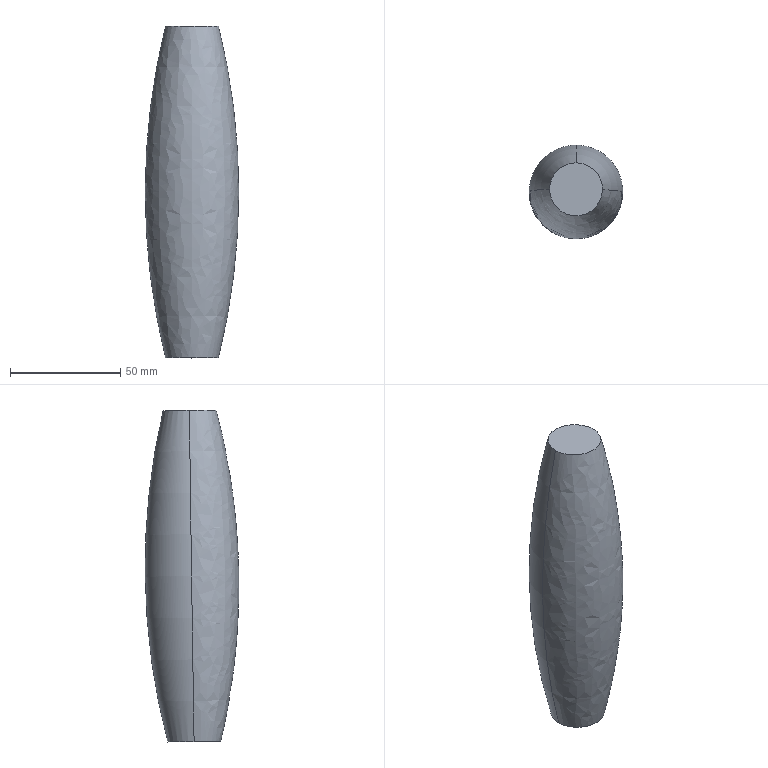Part | SolidWorks | features BaseBody 1 | 1 solid | 5 faces | box 42.361 x 42.419 x 150.325 mm | volume 158549 mm3 | torus 2 | plane 2 | spline 1
STEP:
#1=CARTESIAN_POINT('',(141.643,205.367,-31.785));
#2=VERTEX_POINT('',#1);
#3=CARTESIAN_POINT('',(129.643,193.467,-31.614));
#4=VERTEX_POINT('',#3);
#5=CARTESIAN_POINT('',(141.643,193.368,-31.615));
#6=DIRECTION('',(0.0001428,0.01416,0.9999));
#7=DIRECTION('',(1.,-0.00828,-0.00002558));
#8=AXIS2_PLACEMENT_3D('',#5,#6,#7);
#9=CIRCLE('',#8,12.);
#10=EDGE_CURVE('',#2,#4,#9,.T.);
#11=ORIENTED_EDGE('',*,*,#10,.F.);
#12=CARTESIAN_POINT('',(141.622,203.243,-181.77));
#13=VERTEX_POINT('',#12);
#14=CARTESIAN_POINT('',(141.632,-97.429,-102.504));
#15=DIRECTION('',(-1.,0.000002023,0.0001428));
#16=DIRECTION('',(0.0001428,0.,1.));
#17=AXIS2_PLACEMENT_3D('',#14,#15,#16);
#18=CIRCLE('',#17,310.945);
#19=EDGE_CURVE('',#2,#13,#18,.T.);
#20=ORIENTED_EDGE('',*,*,#19,.T.);
#21=CARTESIAN_POINT('',(129.622,191.343,-181.599));
#22=VERTEX_POINT('',#21);
#23=CARTESIAN_POINT('',(141.622,191.244,-181.6));
#24=DIRECTION('',(-0.0001428,-0.01416,-0.9999));
#25=DIRECTION('',(-1.,0.00828,0.00002558));
#26=AXIS2_PLACEMENT_3D('',#23,#24,#25);
#27=CIRCLE('',#26,12.);
#28=EDGE_CURVE('',#22,#13,#27,.T.);
#29=ORIENTED_EDGE('',*,*,#28,.F.);
#30=CARTESIAN_POINT('',(431.387,189.907,-106.615));
#31=DIRECTION('',(-0.008279,-0.9999,0.01416));
#32=DIRECTION('',(-0.9704,0.01145,0.2412));
#33=AXIS2_PLACEMENT_3D('',#30,#31,#32);
#34=CIRCLE('',#33,310.945);
#35=EDGE_CURVE('',#4,#22,#34,.T.);
#36=ORIENTED_EDGE('',*,*,#35,.F.);
#37=EDGE_LOOP('',(#11,#20,#29,#36));
#38=FACE_OUTER_BOUND('',#37,.T.);
#39=CARTESIAN_POINT('',(141.632,192.306,-106.607));
#40=DIRECTION('',(-0.0001428,-0.01416,-0.9999));
#41=DIRECTION('',(0.,0.9999,-0.01416));
#42=AXIS2_PLACEMENT_3D('',#39,#40,#41);
#43=TOROIDAL_SURFACE('',#42,-289.764,310.945);
#44=ADVANCED_FACE('',(#38),#43,.T.);
#45=ORIENTED_EDGE('',*,*,#28,.T.);
#46=CARTESIAN_POINT('',(153.621,191.145,-181.6));
#47=VERTEX_POINT('',#46);
#48=CARTESIAN_POINT('',(141.622,191.244,-181.6));
#49=DIRECTION('',(-0.0001428,-0.01416,-0.9999));
#50=DIRECTION('',(-1.,0.00828,0.00002558));
#51=AXIS2_PLACEMENT_3D('',#48,#49,#50);
#52=CIRCLE('',#51,12.);
#53=EDGE_CURVE('',#13,#47,#52,.T.);
#54=ORIENTED_EDGE('',*,*,#53,.T.);
#55=CARTESIAN_POINT('',(141.622,191.244,-181.6));
#56=DIRECTION('',(-0.0001428,-0.01416,-0.9999));
#57=DIRECTION('',(1.,-0.00828,-0.00002558));
#58=AXIS2_PLACEMENT_3D('',#55,#56,#57);
#59=CIRCLE('',#58,12.);
#60=EDGE_CURVE('',#47,#22,#59,.T.);
#61=ORIENTED_EDGE('',*,*,#60,.T.);
#62=EDGE_LOOP('',(#45,#54,#61));
#63=FACE_OUTER_BOUND('',#62,.T.);
#64=CARTESIAN_POINT('',(129.622,191.343,-181.599));
#65=DIRECTION('',(0.0001428,0.01416,0.9999));
#66=DIRECTION('',(0.9999,-0.01009,0.));
#67=AXIS2_PLACEMENT_3D('',#64,#65,#66);
#68=PLANE('',#67);
#69=ADVANCED_FACE('',(#63),#68,.F.);
#70=ORIENTED_EDGE('',*,*,#35,.T.);
#71=ORIENTED_EDGE('',*,*,#60,.F.);
#72=CARTESIAN_POINT('',(153.643,193.269,-31.615));
#73=VERTEX_POINT('',#72);
#74=CARTESIAN_POINT('',(-148.122,194.705,-106.6));
#75=DIRECTION('',(0.008279,0.9999,-0.01416));
#76=DIRECTION('',(0.9705,-0.00462,0.2412));
#77=AXIS2_PLACEMENT_3D('',#74,#75,#76);
#78=CIRCLE('',#77,310.945);
#79=EDGE_CURVE('',#73,#47,#78,.T.);
#80=ORIENTED_EDGE('',*,*,#79,.F.);
#81=CARTESIAN_POINT('',(141.643,193.368,-31.615));
#82=DIRECTION('',(0.0001428,0.01416,0.9999));
#83=DIRECTION('',(-1.,0.00828,0.00002558));
#84=AXIS2_PLACEMENT_3D('',#81,#82,#83);
#85=CIRCLE('',#84,12.);
#86=EDGE_CURVE('',#4,#73,#85,.T.);
#87=ORIENTED_EDGE('',*,*,#86,.F.);
#88=EDGE_LOOP('',(#70,#71,#80,#87));
#89=FACE_OUTER_BOUND('',#88,.T.);
#90=CARTESIAN_POINT('',(152.882,194.023,-28.688));
#91=CARTESIAN_POINT('',(166.161,194.021,-80.088));
#92=CARTESIAN_POINT('',(166.153,193.269,-133.171));
#93=CARTESIAN_POINT('',(152.859,191.816,-184.546));
#94=CARTESIAN_POINT('',(153.259,187.108,-28.59));
#95=CARTESIAN_POINT('',(166.985,178.93,-79.875));
#96=CARTESIAN_POINT('',(166.977,178.178,-132.957));
#97=CARTESIAN_POINT('',(153.237,184.901,-184.449));
#98=CARTESIAN_POINT('',(148.476,182.099,-28.519));
#99=CARTESIAN_POINT('',(156.547,167.999,-79.719));
#100=CARTESIAN_POINT('',(156.54,167.247,-132.801));
#101=CARTESIAN_POINT('',(148.454,179.892,-184.377));
#102=CARTESIAN_POINT('',(141.55,182.156,-28.519));
#103=CARTESIAN_POINT('',(141.433,168.124,-79.718));
#104=CARTESIAN_POINT('',(141.425,167.372,-132.8));
#105=CARTESIAN_POINT('',(141.528,179.949,-184.377));
#106=CARTESIAN_POINT('',(134.624,182.214,-28.518));
#107=CARTESIAN_POINT('',(126.319,168.249,-79.718));
#108=CARTESIAN_POINT('',(126.311,167.498,-132.8));
#109=CARTESIAN_POINT('',(134.602,180.006,-184.377));
#110=CARTESIAN_POINT('',(129.925,187.301,-28.59));
#111=CARTESIAN_POINT('',(116.063,179.352,-79.874));
#112=CARTESIAN_POINT('',(116.056,178.6,-132.956));
#113=CARTESIAN_POINT('',(129.903,185.094,-184.448));
#114=CARTESIAN_POINT('',(130.417,194.209,-28.688));
#115=CARTESIAN_POINT('',(117.137,194.427,-80.087));
#116=CARTESIAN_POINT('',(117.13,193.675,-133.17));
#117=CARTESIAN_POINT('',(130.395,192.002,-184.546));
#118=(BOUNDED_SURFACE()B_SPLINE_SURFACE(3,3,((#90,#91,#92,#93),(#94,#95,#96,#97),(#98,#99,#100,#101),(#102,#103,#104,#105),(#106,#107,#108,#109),(#110,#111,#112,#113),(#114,#115,#116,#117)),.UNSPECIFIED.,.F.,.F.,.F.)B_SPLINE_SURFACE_WITH_KNOTS((4,3,4),(4,4),(0.,1.,2.),(0.,1.),.UNSPECIFIED.)GEOMETRIC_REPRESENTATION_ITEM()RATIONAL_B_SPLINE_SURFACE(((1.207,1.181,1.181,1.207),(0.9528,0.9325,0.9325,0.9528),(0.9528,0.9325,0.9325,0.9528),(1.207,1.181,1.181,1.207),(0.9528,0.9325,0.9325,0.9528),(0.9528,0.9325,0.9325,0.9528),(1.207,1.181,1.181,1.207)))REPRESENTATION_ITEM('')SURFACE());
#119=ADVANCED_FACE('',(#89),#118,.T.);
#120=ORIENTED_EDGE('',*,*,#86,.T.);
#121=CARTESIAN_POINT('',(141.643,193.368,-31.615));
#122=DIRECTION('',(0.0001428,0.01416,0.9999));
#123=DIRECTION('',(1.,-0.00828,-0.00002558));
#124=AXIS2_PLACEMENT_3D('',#121,#122,#123);
#125=CIRCLE('',#124,12.);
#126=EDGE_CURVE('',#73,#2,#125,.T.);
#127=ORIENTED_EDGE('',*,*,#126,.T.);
#128=ORIENTED_EDGE('',*,*,#10,.T.);
#129=EDGE_LOOP('',(#120,#127,#128));
#130=FACE_OUTER_BOUND('',#129,.T.);
#131=CARTESIAN_POINT('',(141.643,193.368,-31.615));
#132=DIRECTION('',(-0.0001428,-0.01416,-0.9999));
#133=DIRECTION('',(0.,-0.9999,0.01416));
#134=AXIS2_PLACEMENT_3D('',#131,#132,#133);
#135=PLANE('',#134);
#136=ADVANCED_FACE('',(#130),#135,.F.);
#137=ORIENTED_EDGE('',*,*,#19,.F.);
#138=ORIENTED_EDGE('',*,*,#126,.F.);
#139=ORIENTED_EDGE('',*,*,#79,.T.);
#140=ORIENTED_EDGE('',*,*,#53,.F.);
#141=EDGE_LOOP('',(#137,#138,#139,#140));
#142=FACE_OUTER_BOUND('',#141,.T.);
#143=CARTESIAN_POINT('',(141.632,192.306,-106.607));
#144=DIRECTION('',(-0.0001428,-0.01416,-0.9999));
#145=DIRECTION('',(0.,0.9999,-0.01416));
#146=AXIS2_PLACEMENT_3D('',#143,#144,#145);
#147=TOROIDAL_SURFACE('',#146,-289.764,310.945);
#148=ADVANCED_FACE('',(#142),#147,.T.);
#149=CLOSED_SHELL('',(#44,#69,#119,#136,#148));
#150=MANIFOLD_SOLID_BREP('',#149);
#151=CARTESIAN_POINT('',(0.,0.,0.));
#152=DIRECTION('',(0.,0.,1.));
#153=DIRECTION('',(1.,0.,0.));
#154=AXIS2_PLACEMENT_3D('',#151,#152,#153);
#155=(LENGTH_UNIT()NAMED_UNIT(*)SI_UNIT(.MILLI.,.METRE.));
#156=UNCERTAINTY_MEASURE_WITH_UNIT(LENGTH_MEASURE(0.00001),#155,'','');
#157=(NAMED_UNIT(*)PLANE_ANGLE_UNIT()SI_UNIT($,.RADIAN.));
#158=(NAMED_UNIT(*)SI_UNIT($,.STERADIAN.)SOLID_ANGLE_UNIT());
#159=(GEOMETRIC_REPRESENTATION_CONTEXT(3)GLOBAL_UNCERTAINTY_ASSIGNED_CONTEXT((#156))GLOBAL_UNIT_ASSIGNED_CONTEXT((#155,#157,#158))REPRESENTATION_CONTEXT('',''));
#160=ADVANCED_BREP_SHAPE_REPRESENTATION('',(#150,#154),#159);